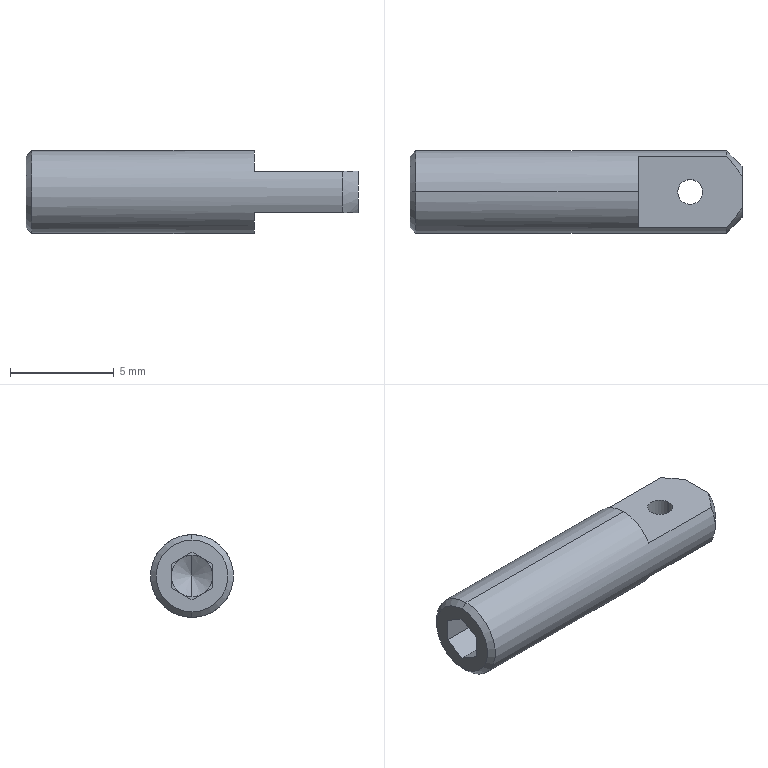Part | STEP file | 1 solid | 28 faces | box 16 x 4 x 4 mm | volume 166.849 mm3 | plane 18 | cone 6 | cylinder 4 | commonest cylinder face diameters 1.2 x2 4 x2